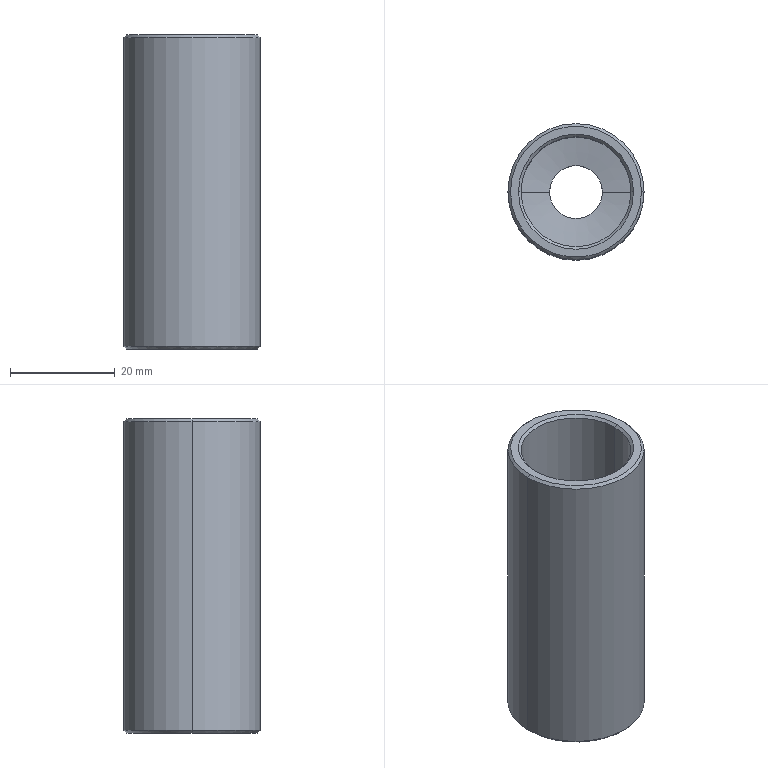Part | STEP file | 31 | 1 solid | 18 faces | box 26 x 26 x 60 mm | volume 14379 mm3 | cone 10 | cylinder 6 | plane 2 | commonest cylinder face diameters 10.106 x2 21 x2 26 x2
STEP:
#1=CARTESIAN_POINT('',(0.,0.,0.));
#2=DIRECTION('',(0.,0.,1.));
#3=DIRECTION('',(1.,0.,0.));
#4=AXIS2_PLACEMENT_3D('',#1,#2,#3);
#5=CARTESIAN_POINT('',(-116.,-78.,75.5));
#6=VERTEX_POINT('',#5);
#7=CARTESIAN_POINT('',(-90.,-78.,75.5));
#8=VERTEX_POINT('',#7);
#9=CARTESIAN_POINT('',(-103.,-78.,75.5));
#10=DIRECTION('',(0.,0.,-1.));
#11=DIRECTION('',(-1.,0.,0.));
#12=AXIS2_PLACEMENT_3D('',#9,#10,#11);
#13=CIRCLE('',#12,13.);
#14=CARTESIAN_POINT('',(-103.,-78.,46.));
#15=DIRECTION('',(0.,0.,-1.));
#16=DIRECTION('',(-1.,0.,0.));
#17=AXIS2_PLACEMENT_3D('',#14,#15,#16);
#18=CYLINDRICAL_SURFACE('',#17,13.);
#19=CARTESIAN_POINT('',(0.,-29.5));
#20=DIRECTION('',(1.,0.));
#21=VECTOR('',#20,1.);
#22=LINE('',#19,#21);
#23=(GEOMETRIC_REPRESENTATION_CONTEXT(2)PARAMETRIC_REPRESENTATION_CONTEXT()REPRESENTATION_CONTEXT('',''));
#24=DEFINITIONAL_REPRESENTATION('',(#22),#23);
#25=PCURVE('',#18,#24);
#26=CARTESIAN_POINT('',(-103.,-78.,75.5));
#27=DIRECTION('',(0.,0.,-1.));
#28=DIRECTION('',(-1.,0.,0.));
#29=AXIS2_PLACEMENT_3D('',#26,#27,#28);
#30=CONICAL_SURFACE('',#29,13.,0.7854);
#31=CARTESIAN_POINT('',(0.,0.));
#32=DIRECTION('',(1.,0.));
#33=VECTOR('',#32,1.);
#34=LINE('',#31,#33);
#35=(GEOMETRIC_REPRESENTATION_CONTEXT(2)PARAMETRIC_REPRESENTATION_CONTEXT()REPRESENTATION_CONTEXT('',''));
#36=DEFINITIONAL_REPRESENTATION('',(#34),#35);
#37=PCURVE('',#30,#36);
#38=SURFACE_CURVE('',#13,(#25,#37),.PCURVE_S1.);
#39=EDGE_CURVE('',#6,#8,#38,.T.);
#40=ORIENTED_EDGE('',*,*,#39,.T.);
#41=CARTESIAN_POINT('',(-90.,-78.,16.5));
#42=VERTEX_POINT('',#41);
#43=CARTESIAN_POINT('',(-90.,-78.,46.));
#44=DIRECTION('',(0.,0.,-1.));
#45=VECTOR('',#44,1.);
#46=LINE('',#43,#45);
#47=CARTESIAN_POINT('',(3.142,0.));
#48=DIRECTION('',(0.,1.));
#49=VECTOR('',#48,1.);
#50=LINE('',#47,#49);
#51=(GEOMETRIC_REPRESENTATION_CONTEXT(2)PARAMETRIC_REPRESENTATION_CONTEXT()REPRESENTATION_CONTEXT('',''));
#52=DEFINITIONAL_REPRESENTATION('',(#50),#51);
#53=PCURVE('',#18,#52);
#54=CARTESIAN_POINT('',(-103.,-78.,46.));
#55=DIRECTION('',(0.,0.,-1.));
#56=DIRECTION('',(-1.,0.,0.));
#57=AXIS2_PLACEMENT_3D('',#54,#55,#56);
#58=CYLINDRICAL_SURFACE('',#57,13.);
#59=CARTESIAN_POINT('',(3.142,0.));
#60=DIRECTION('',(0.,1.));
#61=VECTOR('',#60,1.);
#62=LINE('',#59,#61);
#63=(GEOMETRIC_REPRESENTATION_CONTEXT(2)PARAMETRIC_REPRESENTATION_CONTEXT()REPRESENTATION_CONTEXT('',''));
#64=DEFINITIONAL_REPRESENTATION('',(#62),#63);
#65=PCURVE('',#58,#64);
#66=SURFACE_CURVE('',#46,(#53,#65),.PCURVE_S1.);
#67=EDGE_CURVE('',#8,#42,#66,.T.);
#68=ORIENTED_EDGE('',*,*,#67,.T.);
#69=CARTESIAN_POINT('',(-116.,-78.,16.5));
#70=VERTEX_POINT('',#69);
#71=CARTESIAN_POINT('',(-103.,-78.,16.5));
#72=DIRECTION('',(0.,0.,1.));
#73=DIRECTION('',(-1.,0.,0.));
#74=AXIS2_PLACEMENT_3D('',#71,#72,#73);
#75=CIRCLE('',#74,13.);
#76=CARTESIAN_POINT('',(6.283,29.5));
#77=DIRECTION('',(-1.,0.));
#78=VECTOR('',#77,1.);
#79=LINE('',#76,#78);
#80=(GEOMETRIC_REPRESENTATION_CONTEXT(2)PARAMETRIC_REPRESENTATION_CONTEXT()REPRESENTATION_CONTEXT('',''));
#81=DEFINITIONAL_REPRESENTATION('',(#79),#80);
#82=PCURVE('',#18,#81);
#83=CARTESIAN_POINT('',(-103.,-78.,16.5));
#84=DIRECTION('',(0.,0.,1.));
#85=DIRECTION('',(1.,0.,0.));
#86=AXIS2_PLACEMENT_3D('',#83,#84,#85);
#87=CONICAL_SURFACE('',#86,13.,0.7854);
#88=CARTESIAN_POINT('',(-3.142,0.));
#89=DIRECTION('',(1.,0.));
#90=VECTOR('',#89,1.);
#91=LINE('',#88,#90);
#92=(GEOMETRIC_REPRESENTATION_CONTEXT(2)PARAMETRIC_REPRESENTATION_CONTEXT()REPRESENTATION_CONTEXT('',''));
#93=DEFINITIONAL_REPRESENTATION('',(#91),#92);
#94=PCURVE('',#87,#93);
#95=SURFACE_CURVE('',#75,(#82,#94),.PCURVE_S1.);
#96=EDGE_CURVE('',#42,#70,#95,.T.);
#97=ORIENTED_EDGE('',*,*,#96,.T.);
#98=CARTESIAN_POINT('',(-116.,-78.,46.));
#99=DIRECTION('',(0.,0.,-1.));
#100=VECTOR('',#99,1.);
#101=LINE('',#98,#100);
#102=CARTESIAN_POINT('',(0.,0.));
#103=DIRECTION('',(0.,1.));
#104=VECTOR('',#103,1.);
#105=LINE('',#102,#104);
#106=(GEOMETRIC_REPRESENTATION_CONTEXT(2)PARAMETRIC_REPRESENTATION_CONTEXT()REPRESENTATION_CONTEXT('',''));
#107=DEFINITIONAL_REPRESENTATION('',(#105),#106);
#108=PCURVE('',#18,#107);
#109=CARTESIAN_POINT('',(6.283,0.));
#110=DIRECTION('',(0.,1.));
#111=VECTOR('',#110,1.);
#112=LINE('',#109,#111);
#113=(GEOMETRIC_REPRESENTATION_CONTEXT(2)PARAMETRIC_REPRESENTATION_CONTEXT()REPRESENTATION_CONTEXT('',''));
#114=DEFINITIONAL_REPRESENTATION('',(#112),#113);
#115=PCURVE('',#58,#114);
#116=SURFACE_CURVE('',#101,(#108,#115),.PCURVE_S1.);
#117=EDGE_CURVE('',#6,#70,#116,.T.);
#118=ORIENTED_EDGE('',*,*,#117,.F.);
#119=EDGE_LOOP('',(#40,#68,#97,#118));
#120=FACE_BOUND('',#119,.T.);
#121=ADVANCED_FACE('',(#120),#18,.T.);
#122=CARTESIAN_POINT('',(-115.5,-78.,76.));
#123=VERTEX_POINT('',#122);
#124=CARTESIAN_POINT('',(-90.5,-78.,76.));
#125=VERTEX_POINT('',#124);
#126=CARTESIAN_POINT('',(-103.,-78.,76.));
#127=DIRECTION('',(0.,0.,-1.));
#128=DIRECTION('',(-1.,0.,0.));
#129=AXIS2_PLACEMENT_3D('',#126,#127,#128);
#130=CIRCLE('',#129,12.5);
#131=CARTESIAN_POINT('',(0.,-0.5));
#132=DIRECTION('',(1.,0.));
#133=VECTOR('',#132,1.);
#134=LINE('',#131,#133);
#135=(GEOMETRIC_REPRESENTATION_CONTEXT(2)PARAMETRIC_REPRESENTATION_CONTEXT()REPRESENTATION_CONTEXT('',''));
#136=DEFINITIONAL_REPRESENTATION('',(#134),#135);
#137=PCURVE('',#30,#136);
#138=CARTESIAN_POINT('',(-103.,-71.5,76.));
#139=DIRECTION('',(0.,0.,1.));
#140=DIRECTION('',(1.,0.,0.));
#141=AXIS2_PLACEMENT_3D('',#138,#139,#140);
#142=PLANE('',#141);
#143=CARTESIAN_POINT('',(-12.5,-6.5));
#144=CARTESIAN_POINT('',(-12.5,15.151));
#145=CARTESIAN_POINT('',(6.25,4.325));
#146=CARTESIAN_POINT('',(25.,-6.5));
#147=CARTESIAN_POINT('',(6.25,-17.325));
#148=CARTESIAN_POINT('',(-12.5,-28.151));
#149=CARTESIAN_POINT('',(-12.5,-6.5));
#150=(BOUNDED_CURVE()B_SPLINE_CURVE(2,(#143,#144,#145,#146,#147,#148,#149),.UNSPECIFIED.,.T.,.F.)B_SPLINE_CURVE_WITH_KNOTS((1,2,2,2,2,1),(-2.094,0.,2.094,4.189,6.283,8.378),.UNSPECIFIED.)CURVE()GEOMETRIC_REPRESENTATION_ITEM()RATIONAL_B_SPLINE_CURVE((1.,0.5,1.,0.5,1.,0.5,1.))REPRESENTATION_ITEM(''));
#151=(GEOMETRIC_REPRESENTATION_CONTEXT(2)PARAMETRIC_REPRESENTATION_CONTEXT()REPRESENTATION_CONTEXT('',''));
#152=DEFINITIONAL_REPRESENTATION('',(#150),#151);
#153=PCURVE('',#142,#152);
#154=SURFACE_CURVE('',#130,(#137,#153),.PCURVE_S1.);
#155=EDGE_CURVE('',#123,#125,#154,.T.);
#156=ORIENTED_EDGE('',*,*,#155,.T.);
#157=CARTESIAN_POINT('',(-90.,-78.,75.5));
#158=DIRECTION('',(0.7071,0.,-0.7071));
#159=VECTOR('',#158,1.);
#160=LINE('',#157,#159);
#161=CARTESIAN_POINT('',(3.142,0.));
#162=DIRECTION('',(0.,1.));
#163=VECTOR('',#162,1.);
#164=LINE('',#161,#163);
#165=(GEOMETRIC_REPRESENTATION_CONTEXT(2)PARAMETRIC_REPRESENTATION_CONTEXT()REPRESENTATION_CONTEXT('',''));
#166=DEFINITIONAL_REPRESENTATION('',(#164),#165);
#167=PCURVE('',#30,#166);
#168=CARTESIAN_POINT('',(-103.,-78.,75.5));
#169=DIRECTION('',(0.,0.,-1.));
#170=DIRECTION('',(-1.,0.,0.));
#171=AXIS2_PLACEMENT_3D('',#168,#169,#170);
#172=CONICAL_SURFACE('',#171,13.,0.7854);
#173=CARTESIAN_POINT('',(3.142,0.));
#174=DIRECTION('',(0.,1.));
#175=VECTOR('',#174,1.);
#176=LINE('',#173,#175);
#177=(GEOMETRIC_REPRESENTATION_CONTEXT(2)PARAMETRIC_REPRESENTATION_CONTEXT()REPRESENTATION_CONTEXT('',''));
#178=DEFINITIONAL_REPRESENTATION('',(#176),#177);
#179=PCURVE('',#172,#178);
#180=SURFACE_CURVE('',#160,(#167,#179),.PCURVE_S1.);
#181=EDGE_CURVE('',#125,#8,#180,.T.);
#182=ORIENTED_EDGE('',*,*,#181,.T.);
#183=ORIENTED_EDGE('',*,*,#39,.F.);
#184=CARTESIAN_POINT('',(-116.,-78.,75.5));
#185=DIRECTION('',(-0.7071,0.,-0.7071));
#186=VECTOR('',#185,1.);
#187=LINE('',#184,#186);
#188=CARTESIAN_POINT('',(0.,0.));
#189=DIRECTION('',(0.,1.));
#190=VECTOR('',#189,1.);
#191=LINE('',#188,#190);
#192=(GEOMETRIC_REPRESENTATION_CONTEXT(2)PARAMETRIC_REPRESENTATION_CONTEXT()REPRESENTATION_CONTEXT('',''));
#193=DEFINITIONAL_REPRESENTATION('',(#191),#192);
#194=PCURVE('',#30,#193);
#195=CARTESIAN_POINT('',(6.283,0.));
#196=DIRECTION('',(0.,1.));
#197=VECTOR('',#196,1.);
#198=LINE('',#195,#197);
#199=(GEOMETRIC_REPRESENTATION_CONTEXT(2)PARAMETRIC_REPRESENTATION_CONTEXT()REPRESENTATION_CONTEXT('',''));
#200=DEFINITIONAL_REPRESENTATION('',(#198),#199);
#201=PCURVE('',#172,#200);
#202=SURFACE_CURVE('',#187,(#194,#201),.PCURVE_S1.);
#203=EDGE_CURVE('',#123,#6,#202,.T.);
#204=ORIENTED_EDGE('',*,*,#203,.F.);
#205=EDGE_LOOP('',(#156,#182,#183,#204));
#206=FACE_BOUND('',#205,.T.);
#207=ADVANCED_FACE('',(#206),#30,.T.);
#208=CARTESIAN_POINT('',(-90.5,-78.,16.));
#209=VERTEX_POINT('',#208);
#210=CARTESIAN_POINT('',(-115.5,-78.,16.));
#211=VERTEX_POINT('',#210);
#212=CARTESIAN_POINT('',(-103.,-78.,16.));
#213=DIRECTION('',(0.,0.,1.));
#214=DIRECTION('',(1.,0.,0.));
#215=AXIS2_PLACEMENT_3D('',#212,#213,#214);
#216=CIRCLE('',#215,12.5);
#217=CARTESIAN_POINT('',(0.,-0.5));
#218=DIRECTION('',(1.,0.));
#219=VECTOR('',#218,1.);
#220=LINE('',#217,#219);
#221=(GEOMETRIC_REPRESENTATION_CONTEXT(2)PARAMETRIC_REPRESENTATION_CONTEXT()REPRESENTATION_CONTEXT('',''));
#222=DEFINITIONAL_REPRESENTATION('',(#220),#221);
#223=PCURVE('',#87,#222);
#224=CARTESIAN_POINT('',(-103.,-71.5,16.));
#225=DIRECTION('',(0.,0.,-1.));
#226=DIRECTION('',(-1.,0.,0.));
#227=AXIS2_PLACEMENT_3D('',#224,#225,#226);
#228=PLANE('',#227);
#229=CARTESIAN_POINT('',(-12.5,-6.5));
#230=CARTESIAN_POINT('',(-12.5,15.151));
#231=CARTESIAN_POINT('',(6.25,4.325));
#232=CARTESIAN_POINT('',(25.,-6.5));
#233=CARTESIAN_POINT('',(6.25,-17.325));
#234=CARTESIAN_POINT('',(-12.5,-28.151));
#235=CARTESIAN_POINT('',(-12.5,-6.5));
#236=(BOUNDED_CURVE()B_SPLINE_CURVE(2,(#229,#230,#231,#232,#233,#234,#235),.UNSPECIFIED.,.T.,.F.)B_SPLINE_CURVE_WITH_KNOTS((1,2,2,2,2,1),(-2.094,0.,2.094,4.189,6.283,8.378),.UNSPECIFIED.)CURVE()GEOMETRIC_REPRESENTATION_ITEM()RATIONAL_B_SPLINE_CURVE((1.,0.5,1.,0.5,1.,0.5,1.))REPRESENTATION_ITEM(''));
#237=(GEOMETRIC_REPRESENTATION_CONTEXT(2)PARAMETRIC_REPRESENTATION_CONTEXT()REPRESENTATION_CONTEXT('',''));
#238=DEFINITIONAL_REPRESENTATION('',(#236),#237);
#239=PCURVE('',#228,#238);
#240=SURFACE_CURVE('',#216,(#223,#239),.PCURVE_S1.);
#241=EDGE_CURVE('',#209,#211,#240,.T.);
#242=ORIENTED_EDGE('',*,*,#241,.T.);
#243=CARTESIAN_POINT('',(-116.,-78.,16.5));
#244=DIRECTION('',(-0.7071,0.,0.7071));
#245=VECTOR('',#244,1.);
#246=LINE('',#243,#245);
#247=CARTESIAN_POINT('',(3.142,0.));
#248=DIRECTION('',(0.,1.));
#249=VECTOR('',#248,1.);
#250=LINE('',#247,#249);
#251=(GEOMETRIC_REPRESENTATION_CONTEXT(2)PARAMETRIC_REPRESENTATION_CONTEXT()REPRESENTATION_CONTEXT('',''));
#252=DEFINITIONAL_REPRESENTATION('',(#250),#251);
#253=PCURVE('',#87,#252);
#254=CARTESIAN_POINT('',(-103.,-78.,16.5));
#255=DIRECTION('',(0.,0.,1.));
#256=DIRECTION('',(1.,0.,0.));
#257=AXIS2_PLACEMENT_3D('',#254,#255,#256);
#258=CONICAL_SURFACE('',#257,13.,0.7854);
#259=CARTESIAN_POINT('',(3.142,0.));
#260=DIRECTION('',(0.,1.));
#261=VECTOR('',#260,1.);
#262=LINE('',#259,#261);
#263=(GEOMETRIC_REPRESENTATION_CONTEXT(2)PARAMETRIC_REPRESENTATION_CONTEXT()REPRESENTATION_CONTEXT('',''));
#264=DEFINITIONAL_REPRESENTATION('',(#262),#263);
#265=PCURVE('',#258,#264);
#266=SURFACE_CURVE('',#246,(#253,#265),.PCURVE_S1.);
#267=EDGE_CURVE('',#211,#70,#266,.T.);
#268=ORIENTED_EDGE('',*,*,#267,.T.);
#269=ORIENTED_EDGE('',*,*,#96,.F.);
#270=CARTESIAN_POINT('',(-90.,-78.,16.5));
#271=DIRECTION('',(0.7071,0.,0.7071));
#272=VECTOR('',#271,1.);
#273=LINE('',#270,#272);
#274=CARTESIAN_POINT('',(0.,0.));
#275=DIRECTION('',(0.,1.));
#276=VECTOR('',#275,1.);
#277=LINE('',#274,#276);
#278=(GEOMETRIC_REPRESENTATION_CONTEXT(2)PARAMETRIC_REPRESENTATION_CONTEXT()REPRESENTATION_CONTEXT('',''));
#279=DEFINITIONAL_REPRESENTATION('',(#277),#278);
#280=PCURVE('',#87,#279);
#281=CARTESIAN_POINT('',(6.283,0.));
#282=DIRECTION('',(0.,1.));
#283=VECTOR('',#282,1.);
#284=LINE('',#281,#283);
#285=(GEOMETRIC_REPRESENTATION_CONTEXT(2)PARAMETRIC_REPRESENTATION_CONTEXT()REPRESENTATION_CONTEXT('',''));
#286=DEFINITIONAL_REPRESENTATION('',(#284),#285);
#287=PCURVE('',#258,#286);
#288=SURFACE_CURVE('',#273,(#280,#287),.PCURVE_S1.);
#289=EDGE_CURVE('',#209,#42,#288,.T.);
#290=ORIENTED_EDGE('',*,*,#289,.F.);
#291=EDGE_LOOP('',(#242,#268,#269,#290));
#292=FACE_BOUND('',#291,.T.);
#293=ADVANCED_FACE('',(#292),#87,.T.);
#294=CARTESIAN_POINT('',(-92.5,-78.,75.5));
#295=VERTEX_POINT('',#294);
#296=CARTESIAN_POINT('',(-92.,-78.,76.));
#297=VERTEX_POINT('',#296);
#298=CARTESIAN_POINT('',(-92.,-78.,76.));
#299=DIRECTION('',(0.7071,0.,0.7071));
#300=VECTOR('',#299,1.);
#301=LINE('',#298,#300);
#302=CARTESIAN_POINT('',(-103.,-78.,76.));
#303=DIRECTION('',(0.,0.,1.));
#304=DIRECTION('',(1.,0.,0.));
#305=AXIS2_PLACEMENT_3D('',#302,#303,#304);
#306=CONICAL_SURFACE('',#305,11.,0.7854);
#307=CARTESIAN_POINT('',(6.283,0.));
#308=DIRECTION('',(0.,1.));
#309=VECTOR('',#308,1.);
#310=LINE('',#307,#309);
#311=(GEOMETRIC_REPRESENTATION_CONTEXT(2)PARAMETRIC_REPRESENTATION_CONTEXT()REPRESENTATION_CONTEXT('',''));
#312=DEFINITIONAL_REPRESENTATION('',(#310),#311);
#313=PCURVE('',#306,#312);
#314=CARTESIAN_POINT('',(-103.,-78.,76.));
#315=DIRECTION('',(0.,0.,1.));
#316=DIRECTION('',(1.,0.,0.));
#317=AXIS2_PLACEMENT_3D('',#314,#315,#316);
#318=CONICAL_SURFACE('',#317,11.,0.7854);
#319=CARTESIAN_POINT('',(0.,0.));
#320=DIRECTION('',(0.,1.));
#321=VECTOR('',#320,1.);
#322=LINE('',#319,#321);
#323=(GEOMETRIC_REPRESENTATION_CONTEXT(2)PARAMETRIC_REPRESENTATION_CONTEXT()REPRESENTATION_CONTEXT('',''));
#324=DEFINITIONAL_REPRESENTATION('',(#322),#323);
#325=PCURVE('',#318,#324);
#326=SURFACE_CURVE('',#301,(#313,#325),.PCURVE_S1.);
#327=EDGE_CURVE('',#295,#297,#326,.T.);
#328=ORIENTED_EDGE('',*,*,#327,.T.);
#329=CARTESIAN_POINT('',(-114.,-78.,76.));
#330=VERTEX_POINT('',#329);
#331=CARTESIAN_POINT('',(-103.,-78.,76.));
#332=DIRECTION('',(0.,0.,-1.));
#333=DIRECTION('',(1.,0.,0.));
#334=AXIS2_PLACEMENT_3D('',#331,#332,#333);
#335=CIRCLE('',#334,11.);
#336=CARTESIAN_POINT('',(6.283,0.));
#337=DIRECTION('',(-1.,0.));
#338=VECTOR('',#337,1.);
#339=LINE('',#336,#338);
#340=(GEOMETRIC_REPRESENTATION_CONTEXT(2)PARAMETRIC_REPRESENTATION_CONTEXT()REPRESENTATION_CONTEXT('',''));
#341=DEFINITIONAL_REPRESENTATION('',(#339),#340);
#342=PCURVE('',#306,#341);
#343=CARTESIAN_POINT('',(11.,-6.5));
#344=CARTESIAN_POINT('',(11.,-25.553));
#345=CARTESIAN_POINT('',(-5.5,-16.026));
#346=CARTESIAN_POINT('',(-22.,-6.5));
#347=CARTESIAN_POINT('',(-5.5,3.026));
#348=CARTESIAN_POINT('',(11.,12.553));
#349=CARTESIAN_POINT('',(11.,-6.5));
#350=(BOUNDED_CURVE()B_SPLINE_CURVE(2,(#343,#344,#345,#346,#347,#348,#349),.UNSPECIFIED.,.T.,.F.)B_SPLINE_CURVE_WITH_KNOTS((1,2,2,2,2,1),(-2.094,0.,2.094,4.189,6.283,8.378),.UNSPECIFIED.)CURVE()GEOMETRIC_REPRESENTATION_ITEM()RATIONAL_B_SPLINE_CURVE((1.,0.5,1.,0.5,1.,0.5,1.))REPRESENTATION_ITEM(''));
#351=(GEOMETRIC_REPRESENTATION_CONTEXT(2)PARAMETRIC_REPRESENTATION_CONTEXT()REPRESENTATION_CONTEXT('',''));
#352=DEFINITIONAL_REPRESENTATION('',(#350),#351);
#353=PCURVE('',#142,#352);
#354=SURFACE_CURVE('',#335,(#342,#353),.PCURVE_S1.);
#355=EDGE_CURVE('',#297,#330,#354,.T.);
#356=ORIENTED_EDGE('',*,*,#355,.T.);
#357=CARTESIAN_POINT('',(-113.5,-78.,75.5));
#358=VERTEX_POINT('',#357);
#359=CARTESIAN_POINT('',(-114.,-78.,76.));
#360=DIRECTION('',(-0.7071,0.,0.7071));
#361=VECTOR('',#360,1.);
#362=LINE('',#359,#361);
#363=CARTESIAN_POINT('',(3.142,0.));
#364=DIRECTION('',(0.,1.));
#365=VECTOR('',#364,1.);
#366=LINE('',#363,#365);
#367=(GEOMETRIC_REPRESENTATION_CONTEXT(2)PARAMETRIC_REPRESENTATION_CONTEXT()REPRESENTATION_CONTEXT('',''));
#368=DEFINITIONAL_REPRESENTATION('',(#366),#367);
#369=PCURVE('',#306,#368);
#370=CARTESIAN_POINT('',(3.142,0.));
#371=DIRECTION('',(0.,1.));
#372=VECTOR('',#371,1.);
#373=LINE('',#370,#372);
#374=(GEOMETRIC_REPRESENTATION_CONTEXT(2)PARAMETRIC_REPRESENTATION_CONTEXT()REPRESENTATION_CONTEXT('',''));
#375=DEFINITIONAL_REPRESENTATION('',(#373),#374);
#376=PCURVE('',#318,#375);
#377=SURFACE_CURVE('',#362,(#369,#376),.PCURVE_S1.);
#378=EDGE_CURVE('',#358,#330,#377,.T.);
#379=ORIENTED_EDGE('',*,*,#378,.F.);
#380=CARTESIAN_POINT('',(-103.,-78.,75.5));
#381=DIRECTION('',(0.,0.,1.));
#382=DIRECTION('',(0.,1.,0.));
#383=AXIS2_PLACEMENT_3D('',#380,#381,#382);
#384=CIRCLE('',#383,10.5);
#385=CARTESIAN_POINT('',(1.571,-0.5));
#386=DIRECTION('',(1.,0.));
#387=VECTOR('',#386,1.);
#388=LINE('',#385,#387);
#389=(GEOMETRIC_REPRESENTATION_CONTEXT(2)PARAMETRIC_REPRESENTATION_CONTEXT()REPRESENTATION_CONTEXT('',''));
#390=DEFINITIONAL_REPRESENTATION('',(#388),#389);
#391=PCURVE('',#306,#390);
#392=CARTESIAN_POINT('',(-103.,-78.,52.25));
#393=DIRECTION('',(0.,0.,-1.));
#394=DIRECTION('',(-1.,0.,0.));
#395=AXIS2_PLACEMENT_3D('',#392,#393,#394);
#396=CYLINDRICAL_SURFACE('',#395,10.5);
#397=CARTESIAN_POINT('',(7.854,-23.25));
#398=DIRECTION('',(-1.,0.));
#399=VECTOR('',#398,1.);
#400=LINE('',#397,#399);
#401=(GEOMETRIC_REPRESENTATION_CONTEXT(2)PARAMETRIC_REPRESENTATION_CONTEXT()REPRESENTATION_CONTEXT('',''));
#402=DEFINITIONAL_REPRESENTATION('',(#400),#401);
#403=PCURVE('',#396,#402);
#404=SURFACE_CURVE('',#384,(#391,#403),.PCURVE_S1.);
#405=EDGE_CURVE('',#358,#295,#404,.T.);
#406=ORIENTED_EDGE('',*,*,#405,.T.);
#407=EDGE_LOOP('',(#328,#356,#379,#406));
#408=FACE_BOUND('',#407,.F.);
#409=ADVANCED_FACE('',(#408),#306,.F.);
#410=CARTESIAN_POINT('',(-108.053,-78.,16.947));
#411=VERTEX_POINT('',#410);
#412=CARTESIAN_POINT('',(-109.,-78.,16.));
#413=VERTEX_POINT('',#412);
#414=CARTESIAN_POINT('',(-109.,-78.,16.));
#415=DIRECTION('',(-0.7071,0.,-0.7071));
#416=VECTOR('',#415,1.);
#417=LINE('',#414,#416);
#418=CARTESIAN_POINT('',(-103.,-78.,16.));
#419=DIRECTION('',(0.,0.,-1.));
#420=DIRECTION('',(-1.,0.,0.));
#421=AXIS2_PLACEMENT_3D('',#418,#419,#420);
#422=CONICAL_SURFACE('',#421,6.,0.7854);
#423=CARTESIAN_POINT('',(6.283,0.));
#424=DIRECTION('',(0.,1.));
#425=VECTOR('',#424,1.);
#426=LINE('',#423,#425);
#427=(GEOMETRIC_REPRESENTATION_CONTEXT(2)PARAMETRIC_REPRESENTATION_CONTEXT()REPRESENTATION_CONTEXT('',''));
#428=DEFINITIONAL_REPRESENTATION('',(#426),#427);
#429=PCURVE('',#422,#428);
#430=CARTESIAN_POINT('',(-103.,-78.,16.));
#431=DIRECTION('',(0.,0.,-1.));
#432=DIRECTION('',(-1.,0.,0.));
#433=AXIS2_PLACEMENT_3D('',#430,#431,#432);
#434=CONICAL_SURFACE('',#433,6.,0.7854);
#435=CARTESIAN_POINT('',(0.,0.));
#436=DIRECTION('',(0.,1.));
#437=VECTOR('',#436,1.);
#438=LINE('',#435,#437);
#439=(GEOMETRIC_REPRESENTATION_CONTEXT(2)PARAMETRIC_REPRESENTATION_CONTEXT()REPRESENTATION_CONTEXT('',''));
#440=DEFINITIONAL_REPRESENTATION('',(#438),#439);
#441=PCURVE('',#434,#440);
#442=SURFACE_CURVE('',#417,(#429,#441),.PCURVE_S1.);
#443=EDGE_CURVE('',#411,#413,#442,.T.);
#444=ORIENTED_EDGE('',*,*,#443,.T.);
#445=CARTESIAN_POINT('',(-97.,-78.,16.));
#446=VERTEX_POINT('',#445);
#447=CARTESIAN_POINT('',(-103.,-78.,16.));
#448=DIRECTION('',(0.,0.,1.));
#449=DIRECTION('',(-1.,0.,0.));
#450=AXIS2_PLACEMENT_3D('',#447,#448,#449);
#451=CIRCLE('',#450,6.);
#452=CARTESIAN_POINT('',(6.283,0.));
#453=DIRECTION('',(-1.,0.));
#454=VECTOR('',#453,1.);
#455=LINE('',#452,#454);
#456=(GEOMETRIC_REPRESENTATION_CONTEXT(2)PARAMETRIC_REPRESENTATION_CONTEXT()REPRESENTATION_CONTEXT('',''));
#457=DEFINITIONAL_REPRESENTATION('',(#455),#456);
#458=PCURVE('',#422,#457);
#459=CARTESIAN_POINT('',(6.,-6.5));
#460=CARTESIAN_POINT('',(6.,-16.892));
#461=CARTESIAN_POINT('',(-3.,-11.696));
#462=CARTESIAN_POINT('',(-12.,-6.5));
#463=CARTESIAN_POINT('',(-3.,-1.304));
#464=CARTESIAN_POINT('',(6.,3.892));
#465=CARTESIAN_POINT('',(6.,-6.5));
#466=(BOUNDED_CURVE()B_SPLINE_CURVE(2,(#459,#460,#461,#462,#463,#464,#465),.UNSPECIFIED.,.T.,.F.)B_SPLINE_CURVE_WITH_KNOTS((1,2,2,2,2,1),(-2.094,0.,2.094,4.189,6.283,8.378),.UNSPECIFIED.)CURVE()GEOMETRIC_REPRESENTATION_ITEM()RATIONAL_B_SPLINE_CURVE((1.,0.5,1.,0.5,1.,0.5,1.))REPRESENTATION_ITEM(''));
#467=(GEOMETRIC_REPRESENTATION_CONTEXT(2)PARAMETRIC_REPRESENTATION_CONTEXT()REPRESENTATION_CONTEXT('',''));
#468=DEFINITIONAL_REPRESENTATION('',(#466),#467);
#469=PCURVE('',#228,#468);
#470=SURFACE_CURVE('',#451,(#458,#469),.PCURVE_S1.);
#471=EDGE_CURVE('',#413,#446,#470,.T.);
#472=ORIENTED_EDGE('',*,*,#471,.T.);
#473=CARTESIAN_POINT('',(-97.947,-78.,16.947));
#474=VERTEX_POINT('',#473);
#475=CARTESIAN_POINT('',(-97.,-78.,16.));
#476=DIRECTION('',(0.7071,0.,-0.7071));
#477=VECTOR('',#476,1.);
#478=LINE('',#475,#477);
#479=CARTESIAN_POINT('',(3.142,0.));
#480=DIRECTION('',(0.,1.));
#481=VECTOR('',#480,1.);
#482=LINE('',#479,#481);
#483=(GEOMETRIC_REPRESENTATION_CONTEXT(2)PARAMETRIC_REPRESENTATION_CONTEXT()REPRESENTATION_CONTEXT('',''));
#484=DEFINITIONAL_REPRESENTATION('',(#482),#483);
#485=PCURVE('',#422,#484);
#486=CARTESIAN_POINT('',(3.142,0.));
#487=DIRECTION('',(0.,1.));
#488=VECTOR('',#487,1.);
#489=LINE('',#486,#488);
#490=(GEOMETRIC_REPRESENTATION_CONTEXT(2)PARAMETRIC_REPRESENTATION_CONTEXT()REPRESENTATION_CONTEXT('',''));
#491=DEFINITIONAL_REPRESENTATION('',(#489),#490);
#492=PCURVE('',#434,#491);
#493=SURFACE_CURVE('',#478,(#485,#492),.PCURVE_S1.);
#494=EDGE_CURVE('',#474,#446,#493,.T.);
#495=ORIENTED_EDGE('',*,*,#494,.F.);
#496=CARTESIAN_POINT('',(-103.,-78.,16.947));
#497=DIRECTION('',(0.,0.,-1.));
#498=DIRECTION('',(0.,1.,0.));
#499=AXIS2_PLACEMENT_3D('',#496,#497,#498);
#500=CIRCLE('',#499,5.053);
#501=CARTESIAN_POINT('',(1.571,-0.947));
#502=DIRECTION('',(1.,0.));
#503=VECTOR('',#502,1.);
#504=LINE('',#501,#503);
#505=(GEOMETRIC_REPRESENTATION_CONTEXT(2)PARAMETRIC_REPRESENTATION_CONTEXT()REPRESENTATION_CONTEXT('',''));
#506=DEFINITIONAL_REPRESENTATION('',(#504),#505);
#507=PCURVE('',#422,#506);
#508=CARTESIAN_POINT('',(-103.,-78.,22.5));
#509=DIRECTION('',(0.,0.,-1.));
#510=DIRECTION('',(-1.,0.,0.));
#511=AXIS2_PLACEMENT_3D('',#508,#509,#510);
#512=CYLINDRICAL_SURFACE('',#511,5.053);
#513=CARTESIAN_POINT('',(1.571,5.553));
#514=DIRECTION('',(1.,0.));
#515=VECTOR('',#514,1.);
#516=LINE('',#513,#515);
#517=(GEOMETRIC_REPRESENTATION_CONTEXT(2)PARAMETRIC_REPRESENTATION_CONTEXT()REPRESENTATION_CONTEXT('',''));
#518=DEFINITIONAL_REPRESENTATION('',(#516),#517);
#519=PCURVE('',#512,#518);
#520=SURFACE_CURVE('',#500,(#507,#519),.PCURVE_S1.);
#521=EDGE_CURVE('',#474,#411,#520,.T.);
#522=ORIENTED_EDGE('',*,*,#521,.T.);
#523=EDGE_LOOP('',(#444,#472,#495,#522));
#524=FACE_BOUND('',#523,.F.);
#525=ADVANCED_FACE('',(#524),#422,.F.);
#526=CARTESIAN_POINT('',(-113.5,-78.,29.));
#527=VERTEX_POINT('',#526);
#528=CARTESIAN_POINT('',(-113.5,-78.,52.25));
#529=DIRECTION('',(0.,0.,-1.));
#530=VECTOR('',#529,1.);
#531=LINE('',#528,#530);
#532=CARTESIAN_POINT('',(6.283,0.));
#533=DIRECTION('',(0.,1.));
#534=VECTOR('',#533,1.);
#535=LINE('',#532,#534);
#536=(GEOMETRIC_REPRESENTATION_CONTEXT(2)PARAMETRIC_REPRESENTATION_CONTEXT()REPRESENTATION_CONTEXT('',''));
#537=DEFINITIONAL_REPRESENTATION('',(#535),#536);
#538=PCURVE('',#396,#537);
#539=CARTESIAN_POINT('',(-103.,-78.,52.25));
#540=DIRECTION('',(0.,0.,-1.));
#541=DIRECTION('',(-1.,0.,0.));
#542=AXIS2_PLACEMENT_3D('',#539,#540,#541);
#543=CYLINDRICAL_SURFACE('',#542,10.5);
#544=CARTESIAN_POINT('',(0.,0.));
#545=DIRECTION('',(0.,1.));
#546=VECTOR('',#545,1.);
#547=LINE('',#544,#546);
#548=(GEOMETRIC_REPRESENTATION_CONTEXT(2)PARAMETRIC_REPRESENTATION_CONTEXT()REPRESENTATION_CONTEXT('',''));
#549=DEFINITIONAL_REPRESENTATION('',(#547),#548);
#550=PCURVE('',#543,#549);
#551=SURFACE_CURVE('',#531,(#538,#550),.PCURVE_S1.);
#552=EDGE_CURVE('',#358,#527,#551,.T.);
#553=ORIENTED_EDGE('',*,*,#552,.T.);
#554=CARTESIAN_POINT('',(-92.5,-78.,29.));
#555=VERTEX_POINT('',#554);
#556=CARTESIAN_POINT('',(-103.,-78.,29.));
#557=DIRECTION('',(0.,0.,1.));
#558=DIRECTION('',(-1.,0.,0.));
#559=AXIS2_PLACEMENT_3D('',#556,#557,#558);
#560=CIRCLE('',#559,10.5);
#561=CARTESIAN_POINT('',(6.283,23.25));
#562=DIRECTION('',(-1.,0.));
#563=VECTOR('',#562,1.);
#564=LINE('',#561,#563);
#565=(GEOMETRIC_REPRESENTATION_CONTEXT(2)PARAMETRIC_REPRESENTATION_CONTEXT()REPRESENTATION_CONTEXT('',''));
#566=DEFINITIONAL_REPRESENTATION('',(#564),#565);
#567=PCURVE('',#396,#566);
#568=CARTESIAN_POINT('',(-103.,-78.,29.));
#569=DIRECTION('',(0.,0.,1.));
#570=DIRECTION('',(1.,0.,0.));
#571=AXIS2_PLACEMENT_3D('',#568,#569,#570);
#572=CONICAL_SURFACE('',#571,10.5,1.399);
#573=CARTESIAN_POINT('',(3.142,0.));
#574=DIRECTION('',(1.,0.));
#575=VECTOR('',#574,1.);
#576=LINE('',#573,#575);
#577=(GEOMETRIC_REPRESENTATION_CONTEXT(2)PARAMETRIC_REPRESENTATION_CONTEXT()REPRESENTATION_CONTEXT('',''));
#578=DEFINITIONAL_REPRESENTATION('',(#576),#577);
#579=PCURVE('',#572,#578);
#580=SURFACE_CURVE('',#560,(#567,#579),.PCURVE_S1.);
#581=EDGE_CURVE('',#527,#555,#580,.T.);
#582=ORIENTED_EDGE('',*,*,#581,.T.);
#583=CARTESIAN_POINT('',(-92.5,-78.,52.25));
#584=DIRECTION('',(0.,0.,-1.));
#585=VECTOR('',#584,1.);
#586=LINE('',#583,#585);
#587=CARTESIAN_POINT('',(3.142,0.));
#588=DIRECTION('',(0.,1.));
#589=VECTOR('',#588,1.);
#590=LINE('',#587,#589);
#591=(GEOMETRIC_REPRESENTATION_CONTEXT(2)PARAMETRIC_REPRESENTATION_CONTEXT()REPRESENTATION_CONTEXT('',''));
#592=DEFINITIONAL_REPRESENTATION('',(#590),#591);
#593=PCURVE('',#396,#592);
#594=CARTESIAN_POINT('',(3.142,0.));
#595=DIRECTION('',(0.,1.));
#596=VECTOR('',#595,1.);
#597=LINE('',#594,#596);
#598=(GEOMETRIC_REPRESENTATION_CONTEXT(2)PARAMETRIC_REPRESENTATION_CONTEXT()REPRESENTATION_CONTEXT('',''));
#599=DEFINITIONAL_REPRESENTATION('',(#597),#598);
#600=PCURVE('',#543,#599);
#601=SURFACE_CURVE('',#586,(#593,#600),.PCURVE_S1.);
#602=EDGE_CURVE('',#295,#555,#601,.T.);
#603=ORIENTED_EDGE('',*,*,#602,.F.);
#604=ORIENTED_EDGE('',*,*,#405,.F.);
#605=EDGE_LOOP('',(#553,#582,#603,#604));
#606=FACE_BOUND('',#605,.F.);
#607=ADVANCED_FACE('',(#606),#396,.F.);
#608=CARTESIAN_POINT('',(-108.053,-78.,28.053));
#609=VERTEX_POINT('',#608);
#610=CARTESIAN_POINT('',(-108.053,-78.,22.5));
#611=DIRECTION('',(0.,0.,-1.));
#612=VECTOR('',#611,1.);
#613=LINE('',#610,#612);
#614=CARTESIAN_POINT('',(6.283,0.));
#615=DIRECTION('',(0.,1.));
#616=VECTOR('',#615,1.);
#617=LINE('',#614,#616);
#618=(GEOMETRIC_REPRESENTATION_CONTEXT(2)PARAMETRIC_REPRESENTATION_CONTEXT()REPRESENTATION_CONTEXT('',''));
#619=DEFINITIONAL_REPRESENTATION('',(#617),#618);
#620=PCURVE('',#512,#619);
#621=CARTESIAN_POINT('',(-103.,-78.,22.5));
#622=DIRECTION('',(0.,0.,-1.));
#623=DIRECTION('',(-1.,0.,0.));
#624=AXIS2_PLACEMENT_3D('',#621,#622,#623);
#625=CYLINDRICAL_SURFACE('',#624,5.053);
#626=CARTESIAN_POINT('',(0.,0.));
#627=DIRECTION('',(0.,1.));
#628=VECTOR('',#627,1.);
#629=LINE('',#626,#628);
#630=(GEOMETRIC_REPRESENTATION_CONTEXT(2)PARAMETRIC_REPRESENTATION_CONTEXT()REPRESENTATION_CONTEXT('',''));
#631=DEFINITIONAL_REPRESENTATION('',(#629),#630);
#632=PCURVE('',#625,#631);
#633=SURFACE_CURVE('',#613,(#620,#632),.PCURVE_S1.);
#634=EDGE_CURVE('',#609,#411,#633,.T.);
#635=ORIENTED_EDGE('',*,*,#634,.T.);
#636=ORIENTED_EDGE('',*,*,#521,.F.);
#637=CARTESIAN_POINT('',(-97.947,-78.,28.053));
#638=VERTEX_POINT('',#637);
#639=CARTESIAN_POINT('',(-97.947,-78.,22.5));
#640=DIRECTION('',(0.,0.,-1.));
#641=VECTOR('',#640,1.);
#642=LINE('',#639,#641);
#643=CARTESIAN_POINT('',(3.142,0.));
#644=DIRECTION('',(0.,1.));
#645=VECTOR('',#644,1.);
#646=LINE('',#643,#645);
#647=(GEOMETRIC_REPRESENTATION_CONTEXT(2)PARAMETRIC_REPRESENTATION_CONTEXT()REPRESENTATION_CONTEXT('',''));
#648=DEFINITIONAL_REPRESENTATION('',(#646),#647);
#649=PCURVE('',#512,#648);
#650=CARTESIAN_POINT('',(3.142,0.));
#651=DIRECTION('',(0.,1.));
#652=VECTOR('',#651,1.);
#653=LINE('',#650,#652);
#654=(GEOMETRIC_REPRESENTATION_CONTEXT(2)PARAMETRIC_REPRESENTATION_CONTEXT()REPRESENTATION_CONTEXT('',''));
#655=DEFINITIONAL_REPRESENTATION('',(#653),#654);
#656=PCURVE('',#625,#655);
#657=SURFACE_CURVE('',#642,(#649,#656),.PCURVE_S1.);
#658=EDGE_CURVE('',#638,#474,#657,.T.);
#659=ORIENTED_EDGE('',*,*,#658,.F.);
#660=CARTESIAN_POINT('',(-103.,-78.,28.053));
#661=DIRECTION('',(0.,0.,-1.));
#662=DIRECTION('',(-1.,0.,0.));
#663=AXIS2_PLACEMENT_3D('',#660,#661,#662);
#664=CIRCLE('',#663,5.053);
#665=CARTESIAN_POINT('',(0.,-5.553));
#666=DIRECTION('',(1.,0.));
#667=VECTOR('',#666,1.);
#668=LINE('',#665,#667);
#669=(GEOMETRIC_REPRESENTATION_CONTEXT(2)PARAMETRIC_REPRESENTATION_CONTEXT()REPRESENTATION_CONTEXT('',''));
#670=DEFINITIONAL_REPRESENTATION('',(#668),#669);
#671=PCURVE('',#512,#670);
#672=CARTESIAN_POINT('',(9.425,-0.947));
#673=DIRECTION('',(-1.,0.));
#674=VECTOR('',#673,1.);
#675=LINE('',#672,#674);
#676=(GEOMETRIC_REPRESENTATION_CONTEXT(2)PARAMETRIC_REPRESENTATION_CONTEXT()REPRESENTATION_CONTEXT('',''));
#677=DEFINITIONAL_REPRESENTATION('',(#675),#676);
#678=PCURVE('',#572,#677);
#679=SURFACE_CURVE('',#664,(#671,#678),.PCURVE_S1.);
#680=EDGE_CURVE('',#638,#609,#679,.T.);
#681=ORIENTED_EDGE('',*,*,#680,.T.);
#682=EDGE_LOOP('',(#635,#636,#659,#681));
#683=FACE_BOUND('',#682,.F.);
#684=ADVANCED_FACE('',(#683),#512,.F.);
#685=CARTESIAN_POINT('',(-92.5,-78.,29.));
#686=DIRECTION('',(0.9852,0.,0.1713));
#687=VECTOR('',#686,1.);
#688=LINE('',#685,#687);
#689=CARTESIAN_POINT('',(6.283,0.));
#690=DIRECTION('',(0.,1.));
#691=VECTOR('',#690,1.);
#692=LINE('',#689,#691);
#693=(GEOMETRIC_REPRESENTATION_CONTEXT(2)PARAMETRIC_REPRESENTATION_CONTEXT()REPRESENTATION_CONTEXT('',''));
#694=DEFINITIONAL_REPRESENTATION('',(#692),#693);
#695=PCURVE('',#572,#694);
#696=CARTESIAN_POINT('',(-103.,-78.,29.));
#697=DIRECTION('',(0.,0.,1.));
#698=DIRECTION('',(1.,0.,0.));
#699=AXIS2_PLACEMENT_3D('',#696,#697,#698);
#700=CONICAL_SURFACE('',#699,10.5,1.399);
#701=CARTESIAN_POINT('',(0.,0.));
#702=DIRECTION('',(0.,1.));
#703=VECTOR('',#702,1.);
#704=LINE('',#701,#703);
#705=(GEOMETRIC_REPRESENTATION_CONTEXT(2)PARAMETRIC_REPRESENTATION_CONTEXT()REPRESENTATION_CONTEXT('',''));
#706=DEFINITIONAL_REPRESENTATION('',(#704),#705);
#707=PCURVE('',#700,#706);
#708=SURFACE_CURVE('',#688,(#695,#707),.PCURVE_S1.);
#709=EDGE_CURVE('',#638,#555,#708,.T.);
#710=ORIENTED_EDGE('',*,*,#709,.T.);
#711=ORIENTED_EDGE('',*,*,#581,.F.);
#712=CARTESIAN_POINT('',(-113.5,-78.,29.));
#713=DIRECTION('',(-0.9852,0.,0.1713));
#714=VECTOR('',#713,1.);
#715=LINE('',#712,#714);
#716=CARTESIAN_POINT('',(3.142,0.));
#717=DIRECTION('',(0.,1.));
#718=VECTOR('',#717,1.);
#719=LINE('',#716,#718);
#720=(GEOMETRIC_REPRESENTATION_CONTEXT(2)PARAMETRIC_REPRESENTATION_CONTEXT()REPRESENTATION_CONTEXT('',''));
#721=DEFINITIONAL_REPRESENTATION('',(#719),#720);
#722=PCURVE('',#572,#721);
#723=CARTESIAN_POINT('',(3.142,0.));
#724=DIRECTION('',(0.,1.));
#725=VECTOR('',#724,1.);
#726=LINE('',#723,#725);
#727=(GEOMETRIC_REPRESENTATION_CONTEXT(2)PARAMETRIC_REPRESENTATION_CONTEXT()REPRESENTATION_CONTEXT('',''));
#728=DEFINITIONAL_REPRESENTATION('',(#726),#727);
#729=PCURVE('',#700,#728);
#730=SURFACE_CURVE('',#715,(#722,#729),.PCURVE_S1.);
#731=EDGE_CURVE('',#609,#527,#730,.T.);
#732=ORIENTED_EDGE('',*,*,#731,.F.);
#733=ORIENTED_EDGE('',*,*,#680,.F.);
#734=EDGE_LOOP('',(#710,#711,#732,#733));
#735=FACE_BOUND('',#734,.F.);
#736=ADVANCED_FACE('',(#735),#572,.F.);
#737=ORIENTED_EDGE('',*,*,#67,.F.);
#738=CARTESIAN_POINT('',(-103.,-78.,75.5));
#739=DIRECTION('',(0.,0.,-1.));
#740=DIRECTION('',(-1.,0.,0.));
#741=AXIS2_PLACEMENT_3D('',#738,#739,#740);
#742=CIRCLE('',#741,13.);
#743=CARTESIAN_POINT('',(0.,-29.5));
#744=DIRECTION('',(1.,0.));
#745=VECTOR('',#744,1.);
#746=LINE('',#743,#745);
#747=(GEOMETRIC_REPRESENTATION_CONTEXT(2)PARAMETRIC_REPRESENTATION_CONTEXT()REPRESENTATION_CONTEXT('',''));
#748=DEFINITIONAL_REPRESENTATION('',(#746),#747);
#749=PCURVE('',#58,#748);
#750=CARTESIAN_POINT('',(0.,0.));
#751=DIRECTION('',(1.,0.));
#752=VECTOR('',#751,1.);
#753=LINE('',#750,#752);
#754=(GEOMETRIC_REPRESENTATION_CONTEXT(2)PARAMETRIC_REPRESENTATION_CONTEXT()REPRESENTATION_CONTEXT('',''));
#755=DEFINITIONAL_REPRESENTATION('',(#753),#754);
#756=PCURVE('',#172,#755);
#757=SURFACE_CURVE('',#742,(#749,#756),.PCURVE_S1.);
#758=EDGE_CURVE('',#8,#6,#757,.T.);
#759=ORIENTED_EDGE('',*,*,#758,.T.);
#760=ORIENTED_EDGE('',*,*,#117,.T.);
#761=CARTESIAN_POINT('',(-103.,-78.,16.5));
#762=DIRECTION('',(0.,0.,1.));
#763=DIRECTION('',(-1.,0.,0.));
#764=AXIS2_PLACEMENT_3D('',#761,#762,#763);
#765=CIRCLE('',#764,13.);
#766=CARTESIAN_POINT('',(6.283,29.5));
#767=DIRECTION('',(-1.,0.));
#768=VECTOR('',#767,1.);
#769=LINE('',#766,#768);
#770=(GEOMETRIC_REPRESENTATION_CONTEXT(2)PARAMETRIC_REPRESENTATION_CONTEXT()REPRESENTATION_CONTEXT('',''));
#771=DEFINITIONAL_REPRESENTATION('',(#769),#770);
#772=PCURVE('',#58,#771);
#773=CARTESIAN_POINT('',(3.142,0.));
#774=DIRECTION('',(1.,0.));
#775=VECTOR('',#774,1.);
#776=LINE('',#773,#775);
#777=(GEOMETRIC_REPRESENTATION_CONTEXT(2)PARAMETRIC_REPRESENTATION_CONTEXT()REPRESENTATION_CONTEXT('',''));
#778=DEFINITIONAL_REPRESENTATION('',(#776),#777);
#779=PCURVE('',#258,#778);
#780=SURFACE_CURVE('',#765,(#772,#779),.PCURVE_S1.);
#781=EDGE_CURVE('',#70,#42,#780,.T.);
#782=ORIENTED_EDGE('',*,*,#781,.T.);
#783=EDGE_LOOP('',(#737,#759,#760,#782));
#784=FACE_BOUND('',#783,.T.);
#785=ADVANCED_FACE('',(#784),#58,.T.);
#786=ORIENTED_EDGE('',*,*,#181,.F.);
#787=CARTESIAN_POINT('',(-103.,-78.,76.));
#788=DIRECTION('',(0.,0.,-1.));
#789=DIRECTION('',(-1.,0.,0.));
#790=AXIS2_PLACEMENT_3D('',#787,#788,#789);
#791=CIRCLE('',#790,12.5);
#792=CARTESIAN_POINT('',(0.,-0.5));
#793=DIRECTION('',(1.,0.));
#794=VECTOR('',#793,1.);
#795=LINE('',#792,#794);
#796=(GEOMETRIC_REPRESENTATION_CONTEXT(2)PARAMETRIC_REPRESENTATION_CONTEXT()REPRESENTATION_CONTEXT('',''));
#797=DEFINITIONAL_REPRESENTATION('',(#795),#796);
#798=PCURVE('',#172,#797);
#799=CARTESIAN_POINT('',(-12.5,-6.5));
#800=CARTESIAN_POINT('',(-12.5,15.151));
#801=CARTESIAN_POINT('',(6.25,4.325));
#802=CARTESIAN_POINT('',(25.,-6.5));
#803=CARTESIAN_POINT('',(6.25,-17.325));
#804=CARTESIAN_POINT('',(-12.5,-28.151));
#805=CARTESIAN_POINT('',(-12.5,-6.5));
#806=(BOUNDED_CURVE()B_SPLINE_CURVE(2,(#799,#800,#801,#802,#803,#804,#805),.UNSPECIFIED.,.T.,.F.)B_SPLINE_CURVE_WITH_KNOTS((1,2,2,2,2,1),(-2.094,0.,2.094,4.189,6.283,8.378),.UNSPECIFIED.)CURVE()GEOMETRIC_REPRESENTATION_ITEM()RATIONAL_B_SPLINE_CURVE((1.,0.5,1.,0.5,1.,0.5,1.))REPRESENTATION_ITEM(''));
#807=(GEOMETRIC_REPRESENTATION_CONTEXT(2)PARAMETRIC_REPRESENTATION_CONTEXT()REPRESENTATION_CONTEXT('',''));
#808=DEFINITIONAL_REPRESENTATION('',(#806),#807);
#809=PCURVE('',#142,#808);
#810=SURFACE_CURVE('',#791,(#798,#809),.PCURVE_S1.);
#811=EDGE_CURVE('',#125,#123,#810,.T.);
#812=ORIENTED_EDGE('',*,*,#811,.T.);
#813=ORIENTED_EDGE('',*,*,#203,.T.);
#814=ORIENTED_EDGE('',*,*,#758,.F.);
#815=EDGE_LOOP('',(#786,#812,#813,#814));
#816=FACE_BOUND('',#815,.T.);
#817=ADVANCED_FACE('',(#816),#172,.T.);
#818=ORIENTED_EDGE('',*,*,#267,.F.);
#819=CARTESIAN_POINT('',(-103.,-78.,16.));
#820=DIRECTION('',(0.,0.,1.));
#821=DIRECTION('',(1.,0.,0.));
#822=AXIS2_PLACEMENT_3D('',#819,#820,#821);
#823=CIRCLE('',#822,12.5);
#824=CARTESIAN_POINT('',(0.,-0.5));
#825=DIRECTION('',(1.,0.));
#826=VECTOR('',#825,1.);
#827=LINE('',#824,#826);
#828=(GEOMETRIC_REPRESENTATION_CONTEXT(2)PARAMETRIC_REPRESENTATION_CONTEXT()REPRESENTATION_CONTEXT('',''));
#829=DEFINITIONAL_REPRESENTATION('',(#827),#828);
#830=PCURVE('',#258,#829);
#831=CARTESIAN_POINT('',(-12.5,-6.5));
#832=CARTESIAN_POINT('',(-12.5,15.151));
#833=CARTESIAN_POINT('',(6.25,4.325));
#834=CARTESIAN_POINT('',(25.,-6.5));
#835=CARTESIAN_POINT('',(6.25,-17.325));
#836=CARTESIAN_POINT('',(-12.5,-28.151));
#837=CARTESIAN_POINT('',(-12.5,-6.5));
#838=(BOUNDED_CURVE()B_SPLINE_CURVE(2,(#831,#832,#833,#834,#835,#836,#837),.UNSPECIFIED.,.T.,.F.)B_SPLINE_CURVE_WITH_KNOTS((1,2,2,2,2,1),(-2.094,0.,2.094,4.189,6.283,8.378),.UNSPECIFIED.)CURVE()GEOMETRIC_REPRESENTATION_ITEM()RATIONAL_B_SPLINE_CURVE((1.,0.5,1.,0.5,1.,0.5,1.))REPRESENTATION_ITEM(''));
#839=(GEOMETRIC_REPRESENTATION_CONTEXT(2)PARAMETRIC_REPRESENTATION_CONTEXT()REPRESENTATION_CONTEXT('',''));
#840=DEFINITIONAL_REPRESENTATION('',(#838),#839);
#841=PCURVE('',#228,#840);
#842=SURFACE_CURVE('',#823,(#830,#841),.PCURVE_S1.);
#843=EDGE_CURVE('',#211,#209,#842,.T.);
#844=ORIENTED_EDGE('',*,*,#843,.T.);
#845=ORIENTED_EDGE('',*,*,#289,.T.);
#846=ORIENTED_EDGE('',*,*,#781,.F.);
#847=EDGE_LOOP('',(#818,#844,#845,#846));
#848=FACE_BOUND('',#847,.T.);
#849=ADVANCED_FACE('',(#848),#258,.T.);
#850=ORIENTED_EDGE('',*,*,#155,.F.);
#851=ORIENTED_EDGE('',*,*,#811,.F.);
#852=EDGE_LOOP('',(#850,#851));
#853=FACE_BOUND('',#852,.T.);
#854=ORIENTED_EDGE('',*,*,#355,.T.);
#855=CARTESIAN_POINT('',(-103.,-78.,76.));
#856=DIRECTION('',(0.,0.,-1.));
#857=DIRECTION('',(1.,0.,0.));
#858=AXIS2_PLACEMENT_3D('',#855,#856,#857);
#859=CIRCLE('',#858,11.);
#860=CARTESIAN_POINT('',(11.,-6.5));
#861=CARTESIAN_POINT('',(11.,-25.553));
#862=CARTESIAN_POINT('',(-5.5,-16.026));
#863=CARTESIAN_POINT('',(-22.,-6.5));
#864=CARTESIAN_POINT('',(-5.5,3.026));
#865=CARTESIAN_POINT('',(11.,12.553));
#866=CARTESIAN_POINT('',(11.,-6.5));
#867=(BOUNDED_CURVE()B_SPLINE_CURVE(2,(#860,#861,#862,#863,#864,#865,#866),.UNSPECIFIED.,.T.,.F.)B_SPLINE_CURVE_WITH_KNOTS((1,2,2,2,2,1),(-2.094,0.,2.094,4.189,6.283,8.378),.UNSPECIFIED.)CURVE()GEOMETRIC_REPRESENTATION_ITEM()RATIONAL_B_SPLINE_CURVE((1.,0.5,1.,0.5,1.,0.5,1.))REPRESENTATION_ITEM(''));
#868=(GEOMETRIC_REPRESENTATION_CONTEXT(2)PARAMETRIC_REPRESENTATION_CONTEXT()REPRESENTATION_CONTEXT('',''));
#869=DEFINITIONAL_REPRESENTATION('',(#867),#868);
#870=PCURVE('',#142,#869);
#871=CARTESIAN_POINT('',(6.283,0.));
#872=DIRECTION('',(-1.,0.));
#873=VECTOR('',#872,1.);
#874=LINE('',#871,#873);
#875=(GEOMETRIC_REPRESENTATION_CONTEXT(2)PARAMETRIC_REPRESENTATION_CONTEXT()REPRESENTATION_CONTEXT('',''));
#876=DEFINITIONAL_REPRESENTATION('',(#874),#875);
#877=PCURVE('',#318,#876);
#878=SURFACE_CURVE('',#859,(#870,#877),.PCURVE_S1.);
#879=EDGE_CURVE('',#330,#297,#878,.T.);
#880=ORIENTED_EDGE('',*,*,#879,.T.);
#881=EDGE_LOOP('',(#854,#880));
#882=FACE_BOUND('',#881,.T.);
#883=ADVANCED_FACE('',(#853,#882),#142,.T.);
#884=ORIENTED_EDGE('',*,*,#241,.F.);
#885=ORIENTED_EDGE('',*,*,#843,.F.);
#886=EDGE_LOOP('',(#884,#885));
#887=FACE_BOUND('',#886,.T.);
#888=ORIENTED_EDGE('',*,*,#471,.T.);
#889=CARTESIAN_POINT('',(-103.,-78.,16.));
#890=DIRECTION('',(0.,0.,1.));
#891=DIRECTION('',(-1.,0.,0.));
#892=AXIS2_PLACEMENT_3D('',#889,#890,#891);
#893=CIRCLE('',#892,6.);
#894=CARTESIAN_POINT('',(6.,-6.5));
#895=CARTESIAN_POINT('',(6.,-16.892));
#896=CARTESIAN_POINT('',(-3.,-11.696));
#897=CARTESIAN_POINT('',(-12.,-6.5));
#898=CARTESIAN_POINT('',(-3.,-1.304));
#899=CARTESIAN_POINT('',(6.,3.892));
#900=CARTESIAN_POINT('',(6.,-6.5));
#901=(BOUNDED_CURVE()B_SPLINE_CURVE(2,(#894,#895,#896,#897,#898,#899,#900),.UNSPECIFIED.,.T.,.F.)B_SPLINE_CURVE_WITH_KNOTS((1,2,2,2,2,1),(-2.094,0.,2.094,4.189,6.283,8.378),.UNSPECIFIED.)CURVE()GEOMETRIC_REPRESENTATION_ITEM()RATIONAL_B_SPLINE_CURVE((1.,0.5,1.,0.5,1.,0.5,1.))REPRESENTATION_ITEM(''));
#902=(GEOMETRIC_REPRESENTATION_CONTEXT(2)PARAMETRIC_REPRESENTATION_CONTEXT()REPRESENTATION_CONTEXT('',''));
#903=DEFINITIONAL_REPRESENTATION('',(#901),#902);
#904=PCURVE('',#228,#903);
#905=CARTESIAN_POINT('',(6.283,0.));
#906=DIRECTION('',(-1.,0.));
#907=VECTOR('',#906,1.);
#908=LINE('',#905,#907);
#909=(GEOMETRIC_REPRESENTATION_CONTEXT(2)PARAMETRIC_REPRESENTATION_CONTEXT()REPRESENTATION_CONTEXT('',''));
#910=DEFINITIONAL_REPRESENTATION('',(#908),#909);
#911=PCURVE('',#434,#910);
#912=SURFACE_CURVE('',#893,(#904,#911),.PCURVE_S1.);
#913=EDGE_CURVE('',#446,#413,#912,.T.);
#914=ORIENTED_EDGE('',*,*,#913,.T.);
#915=EDGE_LOOP('',(#888,#914));
#916=FACE_BOUND('',#915,.T.);
#917=ADVANCED_FACE('',(#887,#916),#228,.T.);
#918=ORIENTED_EDGE('',*,*,#879,.T.);
#919=ORIENTED_EDGE('',*,*,#327,.F.);
#920=CARTESIAN_POINT('',(-103.,-78.,75.5));
#921=DIRECTION('',(0.,0.,1.));
#922=DIRECTION('',(0.,1.,0.));
#923=AXIS2_PLACEMENT_3D('',#920,#921,#922);
#924=CIRCLE('',#923,10.5);
#925=CARTESIAN_POINT('',(-4.712,-0.5));
#926=DIRECTION('',(1.,0.));
#927=VECTOR('',#926,1.);
#928=LINE('',#925,#927);
#929=(GEOMETRIC_REPRESENTATION_CONTEXT(2)PARAMETRIC_REPRESENTATION_CONTEXT()REPRESENTATION_CONTEXT('',''));
#930=DEFINITIONAL_REPRESENTATION('',(#928),#929);
#931=PCURVE('',#318,#930);
#932=CARTESIAN_POINT('',(7.854,-23.25));
#933=DIRECTION('',(-1.,0.));
#934=VECTOR('',#933,1.);
#935=LINE('',#932,#934);
#936=(GEOMETRIC_REPRESENTATION_CONTEXT(2)PARAMETRIC_REPRESENTATION_CONTEXT()REPRESENTATION_CONTEXT('',''));
#937=DEFINITIONAL_REPRESENTATION('',(#935),#936);
#938=PCURVE('',#543,#937);
#939=SURFACE_CURVE('',#924,(#931,#938),.PCURVE_S1.);
#940=EDGE_CURVE('',#295,#358,#939,.T.);
#941=ORIENTED_EDGE('',*,*,#940,.T.);
#942=ORIENTED_EDGE('',*,*,#378,.T.);
#943=EDGE_LOOP('',(#918,#919,#941,#942));
#944=FACE_BOUND('',#943,.F.);
#945=ADVANCED_FACE('',(#944),#318,.F.);
#946=ORIENTED_EDGE('',*,*,#913,.T.);
#947=ORIENTED_EDGE('',*,*,#443,.F.);
#948=CARTESIAN_POINT('',(-103.,-78.,16.947));
#949=DIRECTION('',(0.,0.,-1.));
#950=DIRECTION('',(0.,1.,0.));
#951=AXIS2_PLACEMENT_3D('',#948,#949,#950);
#952=CIRCLE('',#951,5.053);
#953=CARTESIAN_POINT('',(-4.712,-0.947));
#954=DIRECTION('',(1.,0.));
#955=VECTOR('',#954,1.);
#956=LINE('',#953,#955);
#957=(GEOMETRIC_REPRESENTATION_CONTEXT(2)PARAMETRIC_REPRESENTATION_CONTEXT()REPRESENTATION_CONTEXT('',''));
#958=DEFINITIONAL_REPRESENTATION('',(#956),#957);
#959=PCURVE('',#434,#958);
#960=CARTESIAN_POINT('',(-4.712,5.553));
#961=DIRECTION('',(1.,0.));
#962=VECTOR('',#961,1.);
#963=LINE('',#960,#962);
#964=(GEOMETRIC_REPRESENTATION_CONTEXT(2)PARAMETRIC_REPRESENTATION_CONTEXT()REPRESENTATION_CONTEXT('',''));
#965=DEFINITIONAL_REPRESENTATION('',(#963),#964);
#966=PCURVE('',#625,#965);
#967=SURFACE_CURVE('',#952,(#959,#966),.PCURVE_S1.);
#968=EDGE_CURVE('',#411,#474,#967,.T.);
#969=ORIENTED_EDGE('',*,*,#968,.T.);
#970=ORIENTED_EDGE('',*,*,#494,.T.);
#971=EDGE_LOOP('',(#946,#947,#969,#970));
#972=FACE_BOUND('',#971,.F.);
#973=ADVANCED_FACE('',(#972),#434,.F.);
#974=CARTESIAN_POINT('',(-103.,-78.,29.));
#975=DIRECTION('',(0.,0.,1.));
#976=DIRECTION('',(-1.,0.,0.));
#977=AXIS2_PLACEMENT_3D('',#974,#975,#976);
#978=CIRCLE('',#977,10.5);
#979=CARTESIAN_POINT('',(6.283,23.25));
#980=DIRECTION('',(-1.,0.));
#981=VECTOR('',#980,1.);
#982=LINE('',#979,#981);
#983=(GEOMETRIC_REPRESENTATION_CONTEXT(2)PARAMETRIC_REPRESENTATION_CONTEXT()REPRESENTATION_CONTEXT('',''));
#984=DEFINITIONAL_REPRESENTATION('',(#982),#983);
#985=PCURVE('',#543,#984);
#986=CARTESIAN_POINT('',(-3.142,0.));
#987=DIRECTION('',(1.,0.));
#988=VECTOR('',#987,1.);
#989=LINE('',#986,#988);
#990=(GEOMETRIC_REPRESENTATION_CONTEXT(2)PARAMETRIC_REPRESENTATION_CONTEXT()REPRESENTATION_CONTEXT('',''));
#991=DEFINITIONAL_REPRESENTATION('',(#989),#990);
#992=PCURVE('',#700,#991);
#993=SURFACE_CURVE('',#978,(#985,#992),.PCURVE_S1.);
#994=EDGE_CURVE('',#555,#527,#993,.T.);
#995=ORIENTED_EDGE('',*,*,#994,.T.);
#996=ORIENTED_EDGE('',*,*,#552,.F.);
#997=ORIENTED_EDGE('',*,*,#940,.F.);
#998=ORIENTED_EDGE('',*,*,#602,.T.);
#999=EDGE_LOOP('',(#995,#996,#997,#998));
#1000=FACE_BOUND('',#999,.F.);
#1001=ADVANCED_FACE('',(#1000),#543,.F.);
#1002=ORIENTED_EDGE('',*,*,#968,.F.);
#1003=ORIENTED_EDGE('',*,*,#634,.F.);
#1004=CARTESIAN_POINT('',(-103.,-78.,28.053));
#1005=DIRECTION('',(0.,0.,-1.));
#1006=DIRECTION('',(-1.,0.,0.));
#1007=AXIS2_PLACEMENT_3D('',#1004,#1005,#1006);
#1008=CIRCLE('',#1007,5.053);
#1009=CARTESIAN_POINT('',(0.,-5.553));
#1010=DIRECTION('',(1.,0.));
#1011=VECTOR('',#1010,1.);
#1012=LINE('',#1009,#1011);
#1013=(GEOMETRIC_REPRESENTATION_CONTEXT(2)PARAMETRIC_REPRESENTATION_CONTEXT()REPRESENTATION_CONTEXT('',''));
#1014=DEFINITIONAL_REPRESENTATION('',(#1012),#1013);
#1015=PCURVE('',#625,#1014);
#1016=CARTESIAN_POINT('',(3.142,-0.947));
#1017=DIRECTION('',(-1.,0.));
#1018=VECTOR('',#1017,1.);
#1019=LINE('',#1016,#1018);
#1020=(GEOMETRIC_REPRESENTATION_CONTEXT(2)PARAMETRIC_REPRESENTATION_CONTEXT()REPRESENTATION_CONTEXT('',''));
#1021=DEFINITIONAL_REPRESENTATION('',(#1019),#1020);
#1022=PCURVE('',#700,#1021);
#1023=SURFACE_CURVE('',#1008,(#1015,#1022),.PCURVE_S1.);
#1024=EDGE_CURVE('',#609,#638,#1023,.T.);
#1025=ORIENTED_EDGE('',*,*,#1024,.T.);
#1026=ORIENTED_EDGE('',*,*,#658,.T.);
#1027=EDGE_LOOP('',(#1002,#1003,#1025,#1026));
#1028=FACE_BOUND('',#1027,.F.);
#1029=ADVANCED_FACE('',(#1028),#625,.F.);
#1030=ORIENTED_EDGE('',*,*,#994,.F.);
#1031=ORIENTED_EDGE('',*,*,#709,.F.);
#1032=ORIENTED_EDGE('',*,*,#1024,.F.);
#1033=ORIENTED_EDGE('',*,*,#731,.T.);
#1034=EDGE_LOOP('',(#1030,#1031,#1032,#1033));
#1035=FACE_BOUND('',#1034,.F.);
#1036=ADVANCED_FACE('',(#1035),#700,.F.);
#1037=CLOSED_SHELL('',(#121,#207,#293,#409,#525,#607,#684,#736,#785,#817,#849,#883,#917,#945,#973,#1001,#1029,#1036));
#1038=MANIFOLD_SOLID_BREP('',#1037);
#1039=(LENGTH_UNIT()NAMED_UNIT(*)SI_UNIT(.MILLI.,.METRE.));
#1040=UNCERTAINTY_MEASURE_WITH_UNIT(LENGTH_MEASURE(0.0000001),#1039,'','');
#1041=(NAMED_UNIT(*)PLANE_ANGLE_UNIT()SI_UNIT($,.RADIAN.));
#1042=(NAMED_UNIT(*)SI_UNIT($,.STERADIAN.)SOLID_ANGLE_UNIT());
#1043=(GEOMETRIC_REPRESENTATION_CONTEXT(3)GLOBAL_UNCERTAINTY_ASSIGNED_CONTEXT((#1040))GLOBAL_UNIT_ASSIGNED_CONTEXT((#1039,#1041,#1042))REPRESENTATION_CONTEXT('',''));
#1044=ADVANCED_BREP_SHAPE_REPRESENTATION('',(#4,#1038),#1043);